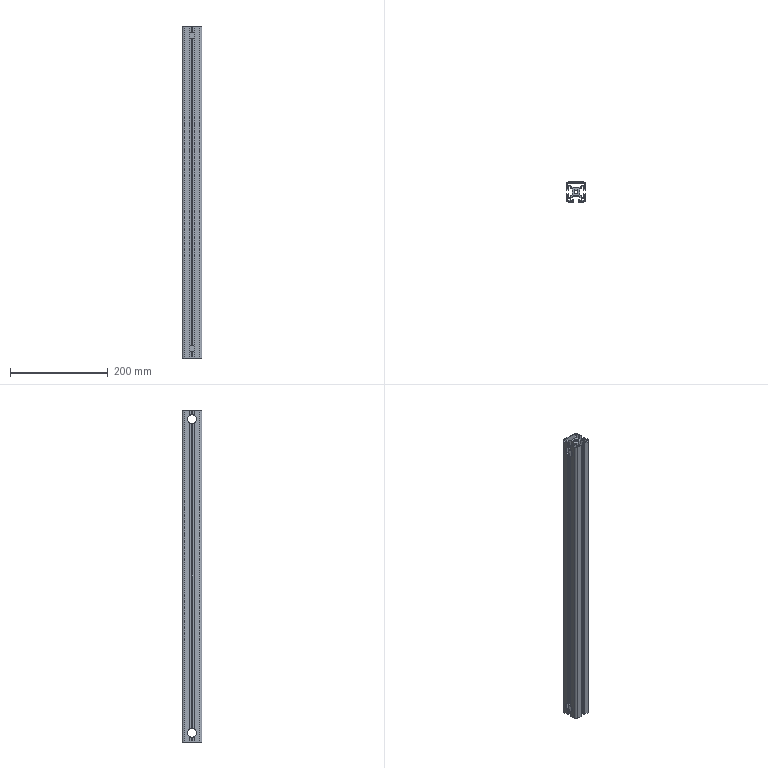Part | SolidWorks | features BaseBody 1, HoleWzd 1, MoveFace 1 | 1 solid | 242 faces | box 40 x 40 x 680 mm | volume 394225 mm3 | plane 187 | cylinder 55 | commonest cylinder face diameters 6.8 x15 2 x14 19 x12 1 x6 5 x4 9 x4